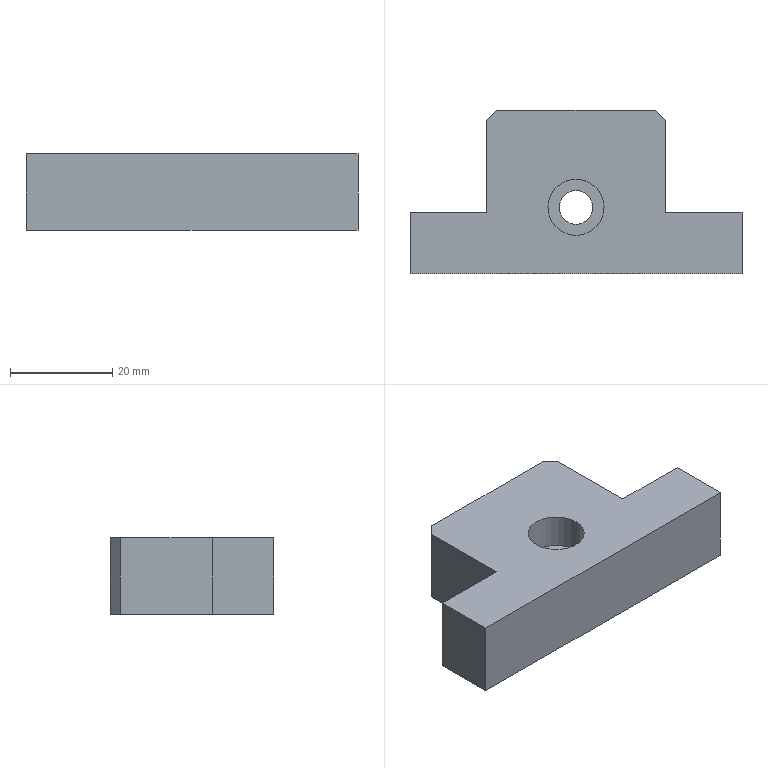Part | STEP file | PN_0005 | 1 solid | 17 faces | box 65 x 32 x 15 mm | volume 21213 mm3 | plane 13 | cylinder 4 | commonest cylinder face diameters 6.6 x2 11 x2
STEP:
#1=CARTESIAN_POINT('',(0.,0.,0.));
#2=DIRECTION('',(0.,0.,1.));
#3=DIRECTION('',(1.,0.,0.));
#4=AXIS2_PLACEMENT_3D('',#1,#2,#3);
#5=CARTESIAN_POINT('',(38.,13.,8.2));
#6=VERTEX_POINT('',#5);
#7=CARTESIAN_POINT('',(38.,13.,15.));
#8=VERTEX_POINT('',#7);
#9=CARTESIAN_POINT('',(38.,13.,15.));
#10=DIRECTION('',(0.,0.,1.));
#11=VECTOR('',#10,1.);
#12=LINE('',#9,#11);
#13=CARTESIAN_POINT('',(32.5,13.,15.));
#14=DIRECTION('',(0.,0.,1.));
#15=DIRECTION('',(1.,0.,0.));
#16=AXIS2_PLACEMENT_3D('',#13,#14,#15);
#17=CYLINDRICAL_SURFACE('',#16,5.5);
#18=CARTESIAN_POINT('',(6.283,0.));
#19=DIRECTION('',(0.,1.));
#20=VECTOR('',#19,1.);
#21=LINE('',#18,#20);
#22=(GEOMETRIC_REPRESENTATION_CONTEXT(2)PARAMETRIC_REPRESENTATION_CONTEXT()REPRESENTATION_CONTEXT('',''));
#23=DEFINITIONAL_REPRESENTATION('',(#21),#22);
#24=PCURVE('',#17,#23);
#25=CARTESIAN_POINT('',(32.5,13.,15.));
#26=DIRECTION('',(0.,0.,1.));
#27=DIRECTION('',(1.,0.,0.));
#28=AXIS2_PLACEMENT_3D('',#25,#26,#27);
#29=CYLINDRICAL_SURFACE('',#28,5.5);
#30=CARTESIAN_POINT('',(0.,0.));
#31=DIRECTION('',(0.,1.));
#32=VECTOR('',#31,1.);
#33=LINE('',#30,#32);
#34=(GEOMETRIC_REPRESENTATION_CONTEXT(2)PARAMETRIC_REPRESENTATION_CONTEXT()REPRESENTATION_CONTEXT('',''));
#35=DEFINITIONAL_REPRESENTATION('',(#33),#34);
#36=PCURVE('',#29,#35);
#37=SURFACE_CURVE('',#12,(#24,#36),.PCURVE_S1.);
#38=EDGE_CURVE('',#6,#8,#37,.T.);
#39=ORIENTED_EDGE('',*,*,#38,.T.);
#40=CARTESIAN_POINT('',(27.,13.,15.));
#41=VERTEX_POINT('',#40);
#42=CARTESIAN_POINT('',(32.5,13.,15.));
#43=DIRECTION('',(0.,0.,1.));
#44=DIRECTION('',(1.,0.,0.));
#45=AXIS2_PLACEMENT_3D('',#42,#43,#44);
#46=CIRCLE('',#45,5.5);
#47=CARTESIAN_POINT('',(0.,0.));
#48=DIRECTION('',(1.,0.));
#49=VECTOR('',#48,1.);
#50=LINE('',#47,#49);
#51=(GEOMETRIC_REPRESENTATION_CONTEXT(2)PARAMETRIC_REPRESENTATION_CONTEXT()REPRESENTATION_CONTEXT('',''));
#52=DEFINITIONAL_REPRESENTATION('',(#50),#51);
#53=PCURVE('',#17,#52);
#54=CARTESIAN_POINT('',(0.,12.,15.));
#55=DIRECTION('',(0.,0.,-1.));
#56=DIRECTION('',(-1.,0.,0.));
#57=AXIS2_PLACEMENT_3D('',#54,#55,#56);
#58=PLANE('',#57);
#59=CARTESIAN_POINT('',(-38.,1.));
#60=CARTESIAN_POINT('',(-38.,10.526));
#61=CARTESIAN_POINT('',(-29.75,5.763));
#62=CARTESIAN_POINT('',(-21.5,1.));
#63=CARTESIAN_POINT('',(-29.75,-3.763));
#64=CARTESIAN_POINT('',(-38.,-8.526));
#65=CARTESIAN_POINT('',(-38.,1.));
#66=(BOUNDED_CURVE()B_SPLINE_CURVE(2,(#59,#60,#61,#62,#63,#64,#65),.UNSPECIFIED.,.T.,.F.)B_SPLINE_CURVE_WITH_KNOTS((1,2,2,2,2,1),(-2.094,0.,2.094,4.189,6.283,8.378),.UNSPECIFIED.)CURVE()GEOMETRIC_REPRESENTATION_ITEM()RATIONAL_B_SPLINE_CURVE((1.,0.5,1.,0.5,1.,0.5,1.))REPRESENTATION_ITEM(''));
#67=(GEOMETRIC_REPRESENTATION_CONTEXT(2)PARAMETRIC_REPRESENTATION_CONTEXT()REPRESENTATION_CONTEXT('',''));
#68=DEFINITIONAL_REPRESENTATION('',(#66),#67);
#69=PCURVE('',#58,#68);
#70=SURFACE_CURVE('',#46,(#53,#69),.PCURVE_S1.);
#71=EDGE_CURVE('',#41,#8,#70,.T.);
#72=ORIENTED_EDGE('',*,*,#71,.F.);
#73=CARTESIAN_POINT('',(27.,13.,8.2));
#74=VERTEX_POINT('',#73);
#75=CARTESIAN_POINT('',(27.,13.,15.));
#76=DIRECTION('',(0.,0.,1.));
#77=VECTOR('',#76,1.);
#78=LINE('',#75,#77);
#79=CARTESIAN_POINT('',(3.142,0.));
#80=DIRECTION('',(0.,1.));
#81=VECTOR('',#80,1.);
#82=LINE('',#79,#81);
#83=(GEOMETRIC_REPRESENTATION_CONTEXT(2)PARAMETRIC_REPRESENTATION_CONTEXT()REPRESENTATION_CONTEXT('',''));
#84=DEFINITIONAL_REPRESENTATION('',(#82),#83);
#85=PCURVE('',#17,#84);
#86=CARTESIAN_POINT('',(3.142,0.));
#87=DIRECTION('',(0.,1.));
#88=VECTOR('',#87,1.);
#89=LINE('',#86,#88);
#90=(GEOMETRIC_REPRESENTATION_CONTEXT(2)PARAMETRIC_REPRESENTATION_CONTEXT()REPRESENTATION_CONTEXT('',''));
#91=DEFINITIONAL_REPRESENTATION('',(#89),#90);
#92=PCURVE('',#29,#91);
#93=SURFACE_CURVE('',#78,(#85,#92),.PCURVE_S1.);
#94=EDGE_CURVE('',#74,#41,#93,.T.);
#95=ORIENTED_EDGE('',*,*,#94,.F.);
#96=CARTESIAN_POINT('',(32.5,13.,8.2));
#97=DIRECTION('',(0.,0.,1.));
#98=DIRECTION('',(1.,0.,0.));
#99=AXIS2_PLACEMENT_3D('',#96,#97,#98);
#100=CIRCLE('',#99,5.5);
#101=CARTESIAN_POINT('',(0.,-6.8));
#102=DIRECTION('',(1.,0.));
#103=VECTOR('',#102,1.);
#104=LINE('',#101,#103);
#105=(GEOMETRIC_REPRESENTATION_CONTEXT(2)PARAMETRIC_REPRESENTATION_CONTEXT()REPRESENTATION_CONTEXT('',''));
#106=DEFINITIONAL_REPRESENTATION('',(#104),#105);
#107=PCURVE('',#17,#106);
#108=CARTESIAN_POINT('',(35.8,13.,8.2));
#109=DIRECTION('',(0.,0.,-1.));
#110=DIRECTION('',(-1.,0.,0.));
#111=AXIS2_PLACEMENT_3D('',#108,#109,#110);
#112=PLANE('',#111);
#113=CARTESIAN_POINT('',(-2.2,0.));
#114=CARTESIAN_POINT('',(-2.2,9.526));
#115=CARTESIAN_POINT('',(6.05,4.763));
#116=CARTESIAN_POINT('',(14.3,0.));
#117=CARTESIAN_POINT('',(6.05,-4.763));
#118=CARTESIAN_POINT('',(-2.2,-9.526));
#119=CARTESIAN_POINT('',(-2.2,0.));
#120=(BOUNDED_CURVE()B_SPLINE_CURVE(2,(#113,#114,#115,#116,#117,#118,#119),.UNSPECIFIED.,.T.,.F.)B_SPLINE_CURVE_WITH_KNOTS((1,2,2,2,2,1),(-2.094,0.,2.094,4.189,6.283,8.378),.UNSPECIFIED.)CURVE()GEOMETRIC_REPRESENTATION_ITEM()RATIONAL_B_SPLINE_CURVE((1.,0.5,1.,0.5,1.,0.5,1.))REPRESENTATION_ITEM(''));
#121=(GEOMETRIC_REPRESENTATION_CONTEXT(2)PARAMETRIC_REPRESENTATION_CONTEXT()REPRESENTATION_CONTEXT('',''));
#122=DEFINITIONAL_REPRESENTATION('',(#120),#121);
#123=PCURVE('',#112,#122);
#124=SURFACE_CURVE('',#100,(#107,#123),.PCURVE_S1.);
#125=EDGE_CURVE('',#74,#6,#124,.T.);
#126=ORIENTED_EDGE('',*,*,#125,.T.);
#127=EDGE_LOOP('',(#39,#72,#95,#126));
#128=FACE_BOUND('',#127,.F.);
#129=ADVANCED_FACE('',(#128),#17,.F.);
#130=CARTESIAN_POINT('',(35.8,13.,0.));
#131=VERTEX_POINT('',#130);
#132=CARTESIAN_POINT('',(35.8,13.,8.2));
#133=VERTEX_POINT('',#132);
#134=CARTESIAN_POINT('',(35.8,13.,15.));
#135=DIRECTION('',(0.,0.,1.));
#136=VECTOR('',#135,1.);
#137=LINE('',#134,#136);
#138=CARTESIAN_POINT('',(32.5,13.,15.));
#139=DIRECTION('',(0.,0.,1.));
#140=DIRECTION('',(1.,0.,0.));
#141=AXIS2_PLACEMENT_3D('',#138,#139,#140);
#142=CYLINDRICAL_SURFACE('',#141,3.3);
#143=CARTESIAN_POINT('',(6.283,0.));
#144=DIRECTION('',(0.,1.));
#145=VECTOR('',#144,1.);
#146=LINE('',#143,#145);
#147=(GEOMETRIC_REPRESENTATION_CONTEXT(2)PARAMETRIC_REPRESENTATION_CONTEXT()REPRESENTATION_CONTEXT('',''));
#148=DEFINITIONAL_REPRESENTATION('',(#146),#147);
#149=PCURVE('',#142,#148);
#150=CARTESIAN_POINT('',(32.5,13.,15.));
#151=DIRECTION('',(0.,0.,1.));
#152=DIRECTION('',(1.,0.,0.));
#153=AXIS2_PLACEMENT_3D('',#150,#151,#152);
#154=CYLINDRICAL_SURFACE('',#153,3.3);
#155=CARTESIAN_POINT('',(0.,0.));
#156=DIRECTION('',(0.,1.));
#157=VECTOR('',#156,1.);
#158=LINE('',#155,#157);
#159=(GEOMETRIC_REPRESENTATION_CONTEXT(2)PARAMETRIC_REPRESENTATION_CONTEXT()REPRESENTATION_CONTEXT('',''));
#160=DEFINITIONAL_REPRESENTATION('',(#158),#159);
#161=PCURVE('',#154,#160);
#162=SURFACE_CURVE('',#137,(#149,#161),.PCURVE_S1.);
#163=EDGE_CURVE('',#131,#133,#162,.T.);
#164=ORIENTED_EDGE('',*,*,#163,.T.);
#165=CARTESIAN_POINT('',(29.2,13.,8.2));
#166=VERTEX_POINT('',#165);
#167=CARTESIAN_POINT('',(32.5,13.,8.2));
#168=DIRECTION('',(0.,0.,1.));
#169=DIRECTION('',(1.,0.,0.));
#170=AXIS2_PLACEMENT_3D('',#167,#168,#169);
#171=CIRCLE('',#170,3.3);
#172=CARTESIAN_POINT('',(0.,-6.8));
#173=DIRECTION('',(1.,0.));
#174=VECTOR('',#173,1.);
#175=LINE('',#172,#174);
#176=(GEOMETRIC_REPRESENTATION_CONTEXT(2)PARAMETRIC_REPRESENTATION_CONTEXT()REPRESENTATION_CONTEXT('',''));
#177=DEFINITIONAL_REPRESENTATION('',(#175),#176);
#178=PCURVE('',#142,#177);
#179=CARTESIAN_POINT('',(0.,0.));
#180=CARTESIAN_POINT('',(0.,5.716));
#181=CARTESIAN_POINT('',(4.95,2.858));
#182=CARTESIAN_POINT('',(9.9,0.));
#183=CARTESIAN_POINT('',(4.95,-2.858));
#184=CARTESIAN_POINT('',(0.,-5.716));
#185=CARTESIAN_POINT('',(0.,0.));
#186=(BOUNDED_CURVE()B_SPLINE_CURVE(2,(#179,#180,#181,#182,#183,#184,#185),.UNSPECIFIED.,.T.,.F.)B_SPLINE_CURVE_WITH_KNOTS((1,2,2,2,2,1),(-2.094,0.,2.094,4.189,6.283,8.378),.UNSPECIFIED.)CURVE()GEOMETRIC_REPRESENTATION_ITEM()RATIONAL_B_SPLINE_CURVE((1.,0.5,1.,0.5,1.,0.5,1.))REPRESENTATION_ITEM(''));
#187=(GEOMETRIC_REPRESENTATION_CONTEXT(2)PARAMETRIC_REPRESENTATION_CONTEXT()REPRESENTATION_CONTEXT('',''));
#188=DEFINITIONAL_REPRESENTATION('',(#186),#187);
#189=PCURVE('',#112,#188);
#190=SURFACE_CURVE('',#171,(#178,#189),.PCURVE_S1.);
#191=EDGE_CURVE('',#166,#133,#190,.T.);
#192=ORIENTED_EDGE('',*,*,#191,.F.);
#193=CARTESIAN_POINT('',(29.2,13.,0.));
#194=VERTEX_POINT('',#193);
#195=CARTESIAN_POINT('',(29.2,13.,15.));
#196=DIRECTION('',(0.,0.,1.));
#197=VECTOR('',#196,1.);
#198=LINE('',#195,#197);
#199=CARTESIAN_POINT('',(3.142,0.));
#200=DIRECTION('',(0.,1.));
#201=VECTOR('',#200,1.);
#202=LINE('',#199,#201);
#203=(GEOMETRIC_REPRESENTATION_CONTEXT(2)PARAMETRIC_REPRESENTATION_CONTEXT()REPRESENTATION_CONTEXT('',''));
#204=DEFINITIONAL_REPRESENTATION('',(#202),#203);
#205=PCURVE('',#142,#204);
#206=CARTESIAN_POINT('',(3.142,0.));
#207=DIRECTION('',(0.,1.));
#208=VECTOR('',#207,1.);
#209=LINE('',#206,#208);
#210=(GEOMETRIC_REPRESENTATION_CONTEXT(2)PARAMETRIC_REPRESENTATION_CONTEXT()REPRESENTATION_CONTEXT('',''));
#211=DEFINITIONAL_REPRESENTATION('',(#209),#210);
#212=PCURVE('',#154,#211);
#213=SURFACE_CURVE('',#198,(#205,#212),.PCURVE_S1.);
#214=EDGE_CURVE('',#194,#166,#213,.T.);
#215=ORIENTED_EDGE('',*,*,#214,.F.);
#216=CARTESIAN_POINT('',(32.5,13.,0.));
#217=DIRECTION('',(0.,0.,1.));
#218=DIRECTION('',(1.,0.,0.));
#219=AXIS2_PLACEMENT_3D('',#216,#217,#218);
#220=CIRCLE('',#219,3.3);
#221=CARTESIAN_POINT('',(0.,-15.));
#222=DIRECTION('',(1.,0.));
#223=VECTOR('',#222,1.);
#224=LINE('',#221,#223);
#225=(GEOMETRIC_REPRESENTATION_CONTEXT(2)PARAMETRIC_REPRESENTATION_CONTEXT()REPRESENTATION_CONTEXT('',''));
#226=DEFINITIONAL_REPRESENTATION('',(#224),#225);
#227=PCURVE('',#142,#226);
#228=CARTESIAN_POINT('',(0.,12.,0.));
#229=DIRECTION('',(0.,0.,-1.));
#230=DIRECTION('',(-1.,0.,0.));
#231=AXIS2_PLACEMENT_3D('',#228,#229,#230);
#232=PLANE('',#231);
#233=CARTESIAN_POINT('',(-35.8,1.));
#234=CARTESIAN_POINT('',(-35.8,6.716));
#235=CARTESIAN_POINT('',(-30.85,3.858));
#236=CARTESIAN_POINT('',(-25.9,1.));
#237=CARTESIAN_POINT('',(-30.85,-1.858));
#238=CARTESIAN_POINT('',(-35.8,-4.716));
#239=CARTESIAN_POINT('',(-35.8,1.));
#240=(BOUNDED_CURVE()B_SPLINE_CURVE(2,(#233,#234,#235,#236,#237,#238,#239),.UNSPECIFIED.,.T.,.F.)B_SPLINE_CURVE_WITH_KNOTS((1,2,2,2,2,1),(-2.094,0.,2.094,4.189,6.283,8.378),.UNSPECIFIED.)CURVE()GEOMETRIC_REPRESENTATION_ITEM()RATIONAL_B_SPLINE_CURVE((1.,0.5,1.,0.5,1.,0.5,1.))REPRESENTATION_ITEM(''));
#241=(GEOMETRIC_REPRESENTATION_CONTEXT(2)PARAMETRIC_REPRESENTATION_CONTEXT()REPRESENTATION_CONTEXT('',''));
#242=DEFINITIONAL_REPRESENTATION('',(#240),#241);
#243=PCURVE('',#232,#242);
#244=SURFACE_CURVE('',#220,(#227,#243),.PCURVE_S1.);
#245=EDGE_CURVE('',#194,#131,#244,.T.);
#246=ORIENTED_EDGE('',*,*,#245,.T.);
#247=EDGE_LOOP('',(#164,#192,#215,#246));
#248=FACE_BOUND('',#247,.F.);
#249=ADVANCED_FACE('',(#248),#142,.F.);
#250=CARTESIAN_POINT('',(0.,12.,0.));
#251=VERTEX_POINT('',#250);
#252=CARTESIAN_POINT('',(0.,0.,0.));
#253=VERTEX_POINT('',#252);
#254=CARTESIAN_POINT('',(0.,0.,0.));
#255=DIRECTION('',(0.,-1.,0.));
#256=VECTOR('',#255,1.);
#257=LINE('',#254,#256);
#258=CARTESIAN_POINT('',(0.,0.,15.));
#259=DIRECTION('',(1.,0.,0.));
#260=DIRECTION('',(0.,0.,-1.));
#261=AXIS2_PLACEMENT_3D('',#258,#259,#260);
#262=PLANE('',#261);
#263=CARTESIAN_POINT('',(15.,0.));
#264=DIRECTION('',(0.,-1.));
#265=VECTOR('',#264,1.);
#266=LINE('',#263,#265);
#267=(GEOMETRIC_REPRESENTATION_CONTEXT(2)PARAMETRIC_REPRESENTATION_CONTEXT()REPRESENTATION_CONTEXT('',''));
#268=DEFINITIONAL_REPRESENTATION('',(#266),#267);
#269=PCURVE('',#262,#268);
#270=CARTESIAN_POINT('',(0.,-12.));
#271=DIRECTION('',(0.,-1.));
#272=VECTOR('',#271,1.);
#273=LINE('',#270,#272);
#274=(GEOMETRIC_REPRESENTATION_CONTEXT(2)PARAMETRIC_REPRESENTATION_CONTEXT()REPRESENTATION_CONTEXT('',''));
#275=DEFINITIONAL_REPRESENTATION('',(#273),#274);
#276=PCURVE('',#232,#275);
#277=SURFACE_CURVE('',#257,(#269,#276),.PCURVE_S1.);
#278=EDGE_CURVE('',#251,#253,#277,.T.);
#279=ORIENTED_EDGE('',*,*,#278,.T.);
#280=CARTESIAN_POINT('',(0.,0.,15.));
#281=VERTEX_POINT('',#280);
#282=CARTESIAN_POINT('',(0.,0.,15.));
#283=DIRECTION('',(0.,0.,-1.));
#284=VECTOR('',#283,1.);
#285=LINE('',#282,#284);
#286=CARTESIAN_POINT('',(0.,0.));
#287=DIRECTION('',(1.,0.));
#288=VECTOR('',#287,1.);
#289=LINE('',#286,#288);
#290=(GEOMETRIC_REPRESENTATION_CONTEXT(2)PARAMETRIC_REPRESENTATION_CONTEXT()REPRESENTATION_CONTEXT('',''));
#291=DEFINITIONAL_REPRESENTATION('',(#289),#290);
#292=PCURVE('',#262,#291);
#293=CARTESIAN_POINT('',(0.,0.,15.));
#294=DIRECTION('',(0.,1.,0.));
#295=DIRECTION('',(-1.,0.,0.));
#296=AXIS2_PLACEMENT_3D('',#293,#294,#295);
#297=PLANE('',#296);
#298=CARTESIAN_POINT('',(0.,0.));
#299=DIRECTION('',(0.,-1.));
#300=VECTOR('',#299,1.);
#301=LINE('',#298,#300);
#302=(GEOMETRIC_REPRESENTATION_CONTEXT(2)PARAMETRIC_REPRESENTATION_CONTEXT()REPRESENTATION_CONTEXT('',''));
#303=DEFINITIONAL_REPRESENTATION('',(#301),#302);
#304=PCURVE('',#297,#303);
#305=SURFACE_CURVE('',#285,(#292,#304),.PCURVE_S1.);
#306=EDGE_CURVE('',#281,#253,#305,.T.);
#307=ORIENTED_EDGE('',*,*,#306,.F.);
#308=CARTESIAN_POINT('',(0.,12.,15.));
#309=VERTEX_POINT('',#308);
#310=CARTESIAN_POINT('',(0.,0.,15.));
#311=DIRECTION('',(0.,-1.,0.));
#312=VECTOR('',#311,1.);
#313=LINE('',#310,#312);
#314=CARTESIAN_POINT('',(0.,0.));
#315=DIRECTION('',(0.,-1.));
#316=VECTOR('',#315,1.);
#317=LINE('',#314,#316);
#318=(GEOMETRIC_REPRESENTATION_CONTEXT(2)PARAMETRIC_REPRESENTATION_CONTEXT()REPRESENTATION_CONTEXT('',''));
#319=DEFINITIONAL_REPRESENTATION('',(#317),#318);
#320=PCURVE('',#262,#319);
#321=CARTESIAN_POINT('',(0.,-12.));
#322=DIRECTION('',(0.,-1.));
#323=VECTOR('',#322,1.);
#324=LINE('',#321,#323);
#325=(GEOMETRIC_REPRESENTATION_CONTEXT(2)PARAMETRIC_REPRESENTATION_CONTEXT()REPRESENTATION_CONTEXT('',''));
#326=DEFINITIONAL_REPRESENTATION('',(#324),#325);
#327=PCURVE('',#58,#326);
#328=SURFACE_CURVE('',#313,(#320,#327),.PCURVE_S1.);
#329=EDGE_CURVE('',#309,#281,#328,.T.);
#330=ORIENTED_EDGE('',*,*,#329,.F.);
#331=CARTESIAN_POINT('',(0.,12.,15.));
#332=DIRECTION('',(0.,0.,-1.));
#333=VECTOR('',#332,1.);
#334=LINE('',#331,#333);
#335=CARTESIAN_POINT('',(0.,12.));
#336=DIRECTION('',(1.,0.));
#337=VECTOR('',#336,1.);
#338=LINE('',#335,#337);
#339=(GEOMETRIC_REPRESENTATION_CONTEXT(2)PARAMETRIC_REPRESENTATION_CONTEXT()REPRESENTATION_CONTEXT('',''));
#340=DEFINITIONAL_REPRESENTATION('',(#338),#339);
#341=PCURVE('',#262,#340);
#342=CARTESIAN_POINT('',(0.,12.,15.));
#343=DIRECTION('',(0.,-1.,0.));
#344=DIRECTION('',(0.,0.,-1.));
#345=AXIS2_PLACEMENT_3D('',#342,#343,#344);
#346=PLANE('',#345);
#347=CARTESIAN_POINT('',(0.,0.));
#348=DIRECTION('',(1.,0.));
#349=VECTOR('',#348,1.);
#350=LINE('',#347,#349);
#351=(GEOMETRIC_REPRESENTATION_CONTEXT(2)PARAMETRIC_REPRESENTATION_CONTEXT()REPRESENTATION_CONTEXT('',''));
#352=DEFINITIONAL_REPRESENTATION('',(#350),#351);
#353=PCURVE('',#346,#352);
#354=SURFACE_CURVE('',#334,(#341,#353),.PCURVE_S1.);
#355=EDGE_CURVE('',#309,#251,#354,.T.);
#356=ORIENTED_EDGE('',*,*,#355,.T.);
#357=EDGE_LOOP('',(#279,#307,#330,#356));
#358=FACE_BOUND('',#357,.T.);
#359=ADVANCED_FACE('',(#358),#262,.F.);
#360=CARTESIAN_POINT('',(65.,0.,0.));
#361=VERTEX_POINT('',#360);
#362=CARTESIAN_POINT('',(0.,0.,0.));
#363=DIRECTION('',(1.,0.,0.));
#364=VECTOR('',#363,1.);
#365=LINE('',#362,#364);
#366=CARTESIAN_POINT('',(0.,-15.));
#367=DIRECTION('',(-1.,0.));
#368=VECTOR('',#367,1.);
#369=LINE('',#366,#368);
#370=(GEOMETRIC_REPRESENTATION_CONTEXT(2)PARAMETRIC_REPRESENTATION_CONTEXT()REPRESENTATION_CONTEXT('',''));
#371=DEFINITIONAL_REPRESENTATION('',(#369),#370);
#372=PCURVE('',#297,#371);
#373=CARTESIAN_POINT('',(0.,-12.));
#374=DIRECTION('',(-1.,0.));
#375=VECTOR('',#374,1.);
#376=LINE('',#373,#375);
#377=(GEOMETRIC_REPRESENTATION_CONTEXT(2)PARAMETRIC_REPRESENTATION_CONTEXT()REPRESENTATION_CONTEXT('',''));
#378=DEFINITIONAL_REPRESENTATION('',(#376),#377);
#379=PCURVE('',#232,#378);
#380=SURFACE_CURVE('',#365,(#372,#379),.PCURVE_S1.);
#381=EDGE_CURVE('',#253,#361,#380,.T.);
#382=ORIENTED_EDGE('',*,*,#381,.T.);
#383=CARTESIAN_POINT('',(65.,0.,15.));
#384=VERTEX_POINT('',#383);
#385=CARTESIAN_POINT('',(65.,0.,15.));
#386=DIRECTION('',(0.,0.,-1.));
#387=VECTOR('',#386,1.);
#388=LINE('',#385,#387);
#389=CARTESIAN_POINT('',(-65.,0.));
#390=DIRECTION('',(0.,-1.));
#391=VECTOR('',#390,1.);
#392=LINE('',#389,#391);
#393=(GEOMETRIC_REPRESENTATION_CONTEXT(2)PARAMETRIC_REPRESENTATION_CONTEXT()REPRESENTATION_CONTEXT('',''));
#394=DEFINITIONAL_REPRESENTATION('',(#392),#393);
#395=PCURVE('',#297,#394);
#396=CARTESIAN_POINT('',(65.,0.,15.));
#397=DIRECTION('',(-1.,0.,0.));
#398=DIRECTION('',(0.,-1.,0.));
#399=AXIS2_PLACEMENT_3D('',#396,#397,#398);
#400=PLANE('',#399);
#401=CARTESIAN_POINT('',(0.,0.));
#402=DIRECTION('',(0.,-1.));
#403=VECTOR('',#402,1.);
#404=LINE('',#401,#403);
#405=(GEOMETRIC_REPRESENTATION_CONTEXT(2)PARAMETRIC_REPRESENTATION_CONTEXT()REPRESENTATION_CONTEXT('',''));
#406=DEFINITIONAL_REPRESENTATION('',(#404),#405);
#407=PCURVE('',#400,#406);
#408=SURFACE_CURVE('',#388,(#395,#407),.PCURVE_S1.);
#409=EDGE_CURVE('',#384,#361,#408,.T.);
#410=ORIENTED_EDGE('',*,*,#409,.F.);
#411=CARTESIAN_POINT('',(0.,0.,15.));
#412=DIRECTION('',(1.,0.,0.));
#413=VECTOR('',#412,1.);
#414=LINE('',#411,#413);
#415=CARTESIAN_POINT('',(0.,0.));
#416=DIRECTION('',(-1.,0.));
#417=VECTOR('',#416,1.);
#418=LINE('',#415,#417);
#419=(GEOMETRIC_REPRESENTATION_CONTEXT(2)PARAMETRIC_REPRESENTATION_CONTEXT()REPRESENTATION_CONTEXT('',''));
#420=DEFINITIONAL_REPRESENTATION('',(#418),#419);
#421=PCURVE('',#297,#420);
#422=CARTESIAN_POINT('',(0.,-12.));
#423=DIRECTION('',(-1.,0.));
#424=VECTOR('',#423,1.);
#425=LINE('',#422,#424);
#426=(GEOMETRIC_REPRESENTATION_CONTEXT(2)PARAMETRIC_REPRESENTATION_CONTEXT()REPRESENTATION_CONTEXT('',''));
#427=DEFINITIONAL_REPRESENTATION('',(#425),#426);
#428=PCURVE('',#58,#427);
#429=SURFACE_CURVE('',#414,(#421,#428),.PCURVE_S1.);
#430=EDGE_CURVE('',#281,#384,#429,.T.);
#431=ORIENTED_EDGE('',*,*,#430,.F.);
#432=ORIENTED_EDGE('',*,*,#306,.T.);
#433=EDGE_LOOP('',(#382,#410,#431,#432));
#434=FACE_BOUND('',#433,.T.);
#435=ADVANCED_FACE('',(#434),#297,.F.);
#436=CARTESIAN_POINT('',(65.,12.,0.));
#437=VERTEX_POINT('',#436);
#438=CARTESIAN_POINT('',(65.,0.,0.));
#439=DIRECTION('',(0.,1.,0.));
#440=VECTOR('',#439,1.);
#441=LINE('',#438,#440);
#442=CARTESIAN_POINT('',(0.,-15.));
#443=DIRECTION('',(-1.,0.));
#444=VECTOR('',#443,1.);
#445=LINE('',#442,#444);
#446=(GEOMETRIC_REPRESENTATION_CONTEXT(2)PARAMETRIC_REPRESENTATION_CONTEXT()REPRESENTATION_CONTEXT('',''));
#447=DEFINITIONAL_REPRESENTATION('',(#445),#446);
#448=PCURVE('',#400,#447);
#449=CARTESIAN_POINT('',(-65.,-12.));
#450=DIRECTION('',(0.,1.));
#451=VECTOR('',#450,1.);
#452=LINE('',#449,#451);
#453=(GEOMETRIC_REPRESENTATION_CONTEXT(2)PARAMETRIC_REPRESENTATION_CONTEXT()REPRESENTATION_CONTEXT('',''));
#454=DEFINITIONAL_REPRESENTATION('',(#452),#453);
#455=PCURVE('',#232,#454);
#456=SURFACE_CURVE('',#441,(#448,#455),.PCURVE_S1.);
#457=EDGE_CURVE('',#361,#437,#456,.T.);
#458=ORIENTED_EDGE('',*,*,#457,.T.);
#459=CARTESIAN_POINT('',(65.,12.,15.));
#460=VERTEX_POINT('',#459);
#461=CARTESIAN_POINT('',(65.,12.,15.));
#462=DIRECTION('',(0.,0.,-1.));
#463=VECTOR('',#462,1.);
#464=LINE('',#461,#463);
#465=CARTESIAN_POINT('',(-12.,0.));
#466=DIRECTION('',(0.,-1.));
#467=VECTOR('',#466,1.);
#468=LINE('',#465,#467);
#469=(GEOMETRIC_REPRESENTATION_CONTEXT(2)PARAMETRIC_REPRESENTATION_CONTEXT()REPRESENTATION_CONTEXT('',''));
#470=DEFINITIONAL_REPRESENTATION('',(#468),#469);
#471=PCURVE('',#400,#470);
#472=CARTESIAN_POINT('',(65.,12.,15.));
#473=DIRECTION('',(0.,-1.,0.));
#474=DIRECTION('',(1.,0.,0.));
#475=AXIS2_PLACEMENT_3D('',#472,#473,#474);
#476=PLANE('',#475);
#477=CARTESIAN_POINT('',(0.,0.));
#478=DIRECTION('',(0.,-1.));
#479=VECTOR('',#478,1.);
#480=LINE('',#477,#479);
#481=(GEOMETRIC_REPRESENTATION_CONTEXT(2)PARAMETRIC_REPRESENTATION_CONTEXT()REPRESENTATION_CONTEXT('',''));
#482=DEFINITIONAL_REPRESENTATION('',(#480),#481);
#483=PCURVE('',#476,#482);
#484=SURFACE_CURVE('',#464,(#471,#483),.PCURVE_S1.);
#485=EDGE_CURVE('',#460,#437,#484,.T.);
#486=ORIENTED_EDGE('',*,*,#485,.F.);
#487=CARTESIAN_POINT('',(65.,0.,15.));
#488=DIRECTION('',(0.,1.,0.));
#489=VECTOR('',#488,1.);
#490=LINE('',#487,#489);
#491=CARTESIAN_POINT('',(0.,0.));
#492=DIRECTION('',(-1.,0.));
#493=VECTOR('',#492,1.);
#494=LINE('',#491,#493);
#495=(GEOMETRIC_REPRESENTATION_CONTEXT(2)PARAMETRIC_REPRESENTATION_CONTEXT()REPRESENTATION_CONTEXT('',''));
#496=DEFINITIONAL_REPRESENTATION('',(#494),#495);
#497=PCURVE('',#400,#496);
#498=CARTESIAN_POINT('',(-65.,-12.));
#499=DIRECTION('',(0.,1.));
#500=VECTOR('',#499,1.);
#501=LINE('',#498,#500);
#502=(GEOMETRIC_REPRESENTATION_CONTEXT(2)PARAMETRIC_REPRESENTATION_CONTEXT()REPRESENTATION_CONTEXT('',''));
#503=DEFINITIONAL_REPRESENTATION('',(#501),#502);
#504=PCURVE('',#58,#503);
#505=SURFACE_CURVE('',#490,(#497,#504),.PCURVE_S1.);
#506=EDGE_CURVE('',#384,#460,#505,.T.);
#507=ORIENTED_EDGE('',*,*,#506,.F.);
#508=ORIENTED_EDGE('',*,*,#409,.T.);
#509=EDGE_LOOP('',(#458,#486,#507,#508));
#510=FACE_BOUND('',#509,.T.);
#511=ADVANCED_FACE('',(#510),#400,.F.);
#512=CARTESIAN_POINT('',(50.,12.,0.));
#513=VERTEX_POINT('',#512);
#514=CARTESIAN_POINT('',(65.,12.,0.));
#515=DIRECTION('',(-1.,0.,0.));
#516=VECTOR('',#515,1.);
#517=LINE('',#514,#516);
#518=CARTESIAN_POINT('',(0.,-15.));
#519=DIRECTION('',(-1.,0.));
#520=VECTOR('',#519,1.);
#521=LINE('',#518,#520);
#522=(GEOMETRIC_REPRESENTATION_CONTEXT(2)PARAMETRIC_REPRESENTATION_CONTEXT()REPRESENTATION_CONTEXT('',''));
#523=DEFINITIONAL_REPRESENTATION('',(#521),#522);
#524=PCURVE('',#476,#523);
#525=CARTESIAN_POINT('',(-65.,0.));
#526=DIRECTION('',(1.,0.));
#527=VECTOR('',#526,1.);
#528=LINE('',#525,#527);
#529=(GEOMETRIC_REPRESENTATION_CONTEXT(2)PARAMETRIC_REPRESENTATION_CONTEXT()REPRESENTATION_CONTEXT('',''));
#530=DEFINITIONAL_REPRESENTATION('',(#528),#529);
#531=PCURVE('',#232,#530);
#532=SURFACE_CURVE('',#517,(#524,#531),.PCURVE_S1.);
#533=EDGE_CURVE('',#437,#513,#532,.T.);
#534=ORIENTED_EDGE('',*,*,#533,.T.);
#535=CARTESIAN_POINT('',(50.,12.,15.));
#536=VERTEX_POINT('',#535);
#537=CARTESIAN_POINT('',(50.,12.,15.));
#538=DIRECTION('',(0.,0.,-1.));
#539=VECTOR('',#538,1.);
#540=LINE('',#537,#539);
#541=CARTESIAN_POINT('',(-15.,0.));
#542=DIRECTION('',(0.,-1.));
#543=VECTOR('',#542,1.);
#544=LINE('',#541,#543);
#545=(GEOMETRIC_REPRESENTATION_CONTEXT(2)PARAMETRIC_REPRESENTATION_CONTEXT()REPRESENTATION_CONTEXT('',''));
#546=DEFINITIONAL_REPRESENTATION('',(#544),#545);
#547=PCURVE('',#476,#546);
#548=CARTESIAN_POINT('',(50.,12.,15.));
#549=DIRECTION('',(-1.,0.,0.));
#550=DIRECTION('',(0.,-1.,0.));
#551=AXIS2_PLACEMENT_3D('',#548,#549,#550);
#552=PLANE('',#551);
#553=CARTESIAN_POINT('',(0.,0.));
#554=DIRECTION('',(0.,-1.));
#555=VECTOR('',#554,1.);
#556=LINE('',#553,#555);
#557=(GEOMETRIC_REPRESENTATION_CONTEXT(2)PARAMETRIC_REPRESENTATION_CONTEXT()REPRESENTATION_CONTEXT('',''));
#558=DEFINITIONAL_REPRESENTATION('',(#556),#557);
#559=PCURVE('',#552,#558);
#560=SURFACE_CURVE('',#540,(#547,#559),.PCURVE_S1.);
#561=EDGE_CURVE('',#536,#513,#560,.T.);
#562=ORIENTED_EDGE('',*,*,#561,.F.);
#563=CARTESIAN_POINT('',(65.,12.,15.));
#564=DIRECTION('',(-1.,0.,0.));
#565=VECTOR('',#564,1.);
#566=LINE('',#563,#565);
#567=CARTESIAN_POINT('',(0.,0.));
#568=DIRECTION('',(-1.,0.));
#569=VECTOR('',#568,1.);
#570=LINE('',#567,#569);
#571=(GEOMETRIC_REPRESENTATION_CONTEXT(2)PARAMETRIC_REPRESENTATION_CONTEXT()REPRESENTATION_CONTEXT('',''));
#572=DEFINITIONAL_REPRESENTATION('',(#570),#571);
#573=PCURVE('',#476,#572);
#574=CARTESIAN_POINT('',(-65.,0.));
#575=DIRECTION('',(1.,0.));
#576=VECTOR('',#575,1.);
#577=LINE('',#574,#576);
#578=(GEOMETRIC_REPRESENTATION_CONTEXT(2)PARAMETRIC_REPRESENTATION_CONTEXT()REPRESENTATION_CONTEXT('',''));
#579=DEFINITIONAL_REPRESENTATION('',(#577),#578);
#580=PCURVE('',#58,#579);
#581=SURFACE_CURVE('',#566,(#573,#580),.PCURVE_S1.);
#582=EDGE_CURVE('',#460,#536,#581,.T.);
#583=ORIENTED_EDGE('',*,*,#582,.F.);
#584=ORIENTED_EDGE('',*,*,#485,.T.);
#585=EDGE_LOOP('',(#534,#562,#583,#584));
#586=FACE_BOUND('',#585,.T.);
#587=ADVANCED_FACE('',(#586),#476,.F.);
#588=CARTESIAN_POINT('',(50.,30.,0.));
#589=VERTEX_POINT('',#588);
#590=CARTESIAN_POINT('',(50.,12.,0.));
#591=DIRECTION('',(0.,1.,0.));
#592=VECTOR('',#591,1.);
#593=LINE('',#590,#592);
#594=CARTESIAN_POINT('',(0.,-15.));
#595=DIRECTION('',(-1.,0.));
#596=VECTOR('',#595,1.);
#597=LINE('',#594,#596);
#598=(GEOMETRIC_REPRESENTATION_CONTEXT(2)PARAMETRIC_REPRESENTATION_CONTEXT()REPRESENTATION_CONTEXT('',''));
#599=DEFINITIONAL_REPRESENTATION('',(#597),#598);
#600=PCURVE('',#552,#599);
#601=CARTESIAN_POINT('',(-50.,0.));
#602=DIRECTION('',(0.,1.));
#603=VECTOR('',#602,1.);
#604=LINE('',#601,#603);
#605=(GEOMETRIC_REPRESENTATION_CONTEXT(2)PARAMETRIC_REPRESENTATION_CONTEXT()REPRESENTATION_CONTEXT('',''));
#606=DEFINITIONAL_REPRESENTATION('',(#604),#605);
#607=PCURVE('',#232,#606);
#608=SURFACE_CURVE('',#593,(#600,#607),.PCURVE_S1.);
#609=EDGE_CURVE('',#513,#589,#608,.T.);
#610=ORIENTED_EDGE('',*,*,#609,.T.);
#611=CARTESIAN_POINT('',(50.,30.,15.));
#612=VERTEX_POINT('',#611);
#613=CARTESIAN_POINT('',(50.,30.,15.));
#614=DIRECTION('',(0.,0.,1.));
#615=VECTOR('',#614,1.);
#616=LINE('',#613,#615);
#617=CARTESIAN_POINT('',(-18.,0.));
#618=DIRECTION('',(0.,1.));
#619=VECTOR('',#618,1.);
#620=LINE('',#617,#619);
#621=(GEOMETRIC_REPRESENTATION_CONTEXT(2)PARAMETRIC_REPRESENTATION_CONTEXT()REPRESENTATION_CONTEXT('',''));
#622=DEFINITIONAL_REPRESENTATION('',(#620),#621);
#623=PCURVE('',#552,#622);
#624=CARTESIAN_POINT('',(48.,32.,15.));
#625=DIRECTION('',(-0.7071,-0.7071,0.));
#626=DIRECTION('',(0.7071,-0.7071,0.));
#627=AXIS2_PLACEMENT_3D('',#624,#625,#626);
#628=PLANE('',#627);
#629=CARTESIAN_POINT('',(2.828,0.));
#630=DIRECTION('',(0.,1.));
#631=VECTOR('',#630,1.);
#632=LINE('',#629,#631);
#633=(GEOMETRIC_REPRESENTATION_CONTEXT(2)PARAMETRIC_REPRESENTATION_CONTEXT()REPRESENTATION_CONTEXT('',''));
#634=DEFINITIONAL_REPRESENTATION('',(#632),#633);
#635=PCURVE('',#628,#634);
#636=SURFACE_CURVE('',#616,(#623,#635),.PCURVE_S1.);
#637=EDGE_CURVE('',#589,#612,#636,.T.);
#638=ORIENTED_EDGE('',*,*,#637,.T.);
#639=CARTESIAN_POINT('',(50.,12.,15.));
#640=DIRECTION('',(0.,1.,0.));
#641=VECTOR('',#640,1.);
#642=LINE('',#639,#641);
#643=CARTESIAN_POINT('',(0.,0.));
#644=DIRECTION('',(-1.,0.));
#645=VECTOR('',#644,1.);
#646=LINE('',#643,#645);
#647=(GEOMETRIC_REPRESENTATION_CONTEXT(2)PARAMETRIC_REPRESENTATION_CONTEXT()REPRESENTATION_CONTEXT('',''));
#648=DEFINITIONAL_REPRESENTATION('',(#646),#647);
#649=PCURVE('',#552,#648);
#650=CARTESIAN_POINT('',(-50.,0.));
#651=DIRECTION('',(0.,1.));
#652=VECTOR('',#651,1.);
#653=LINE('',#650,#652);
#654=(GEOMETRIC_REPRESENTATION_CONTEXT(2)PARAMETRIC_REPRESENTATION_CONTEXT()REPRESENTATION_CONTEXT('',''));
#655=DEFINITIONAL_REPRESENTATION('',(#653),#654);
#656=PCURVE('',#58,#655);
#657=SURFACE_CURVE('',#642,(#649,#656),.PCURVE_S1.);
#658=EDGE_CURVE('',#536,#612,#657,.T.);
#659=ORIENTED_EDGE('',*,*,#658,.F.);
#660=ORIENTED_EDGE('',*,*,#561,.T.);
#661=EDGE_LOOP('',(#610,#638,#659,#660));
#662=FACE_BOUND('',#661,.T.);
#663=ADVANCED_FACE('',(#662),#552,.F.);
#664=CARTESIAN_POINT('',(48.,32.,15.));
#665=VERTEX_POINT('',#664);
#666=CARTESIAN_POINT('',(17.,32.,15.));
#667=VERTEX_POINT('',#666);
#668=CARTESIAN_POINT('',(15.,32.,15.));
#669=DIRECTION('',(-1.,0.,0.));
#670=VECTOR('',#669,1.);
#671=LINE('',#668,#670);
#672=CARTESIAN_POINT('',(15.,32.,15.));
#673=DIRECTION('',(0.,-1.,0.));
#674=DIRECTION('',(1.,0.,0.));
#675=AXIS2_PLACEMENT_3D('',#672,#673,#674);
#676=PLANE('',#675);
#677=CARTESIAN_POINT('',(0.,0.));
#678=DIRECTION('',(-1.,0.));
#679=VECTOR('',#678,1.);
#680=LINE('',#677,#679);
#681=(GEOMETRIC_REPRESENTATION_CONTEXT(2)PARAMETRIC_REPRESENTATION_CONTEXT()REPRESENTATION_CONTEXT('',''));
#682=DEFINITIONAL_REPRESENTATION('',(#680),#681);
#683=PCURVE('',#676,#682);
#684=CARTESIAN_POINT('',(-15.,20.));
#685=DIRECTION('',(1.,0.));
#686=VECTOR('',#685,1.);
#687=LINE('',#684,#686);
#688=(GEOMETRIC_REPRESENTATION_CONTEXT(2)PARAMETRIC_REPRESENTATION_CONTEXT()REPRESENTATION_CONTEXT('',''));
#689=DEFINITIONAL_REPRESENTATION('',(#687),#688);
#690=PCURVE('',#58,#689);
#691=SURFACE_CURVE('',#671,(#683,#690),.PCURVE_S1.);
#692=EDGE_CURVE('',#665,#667,#691,.T.);
#693=ORIENTED_EDGE('',*,*,#692,.F.);
#694=CARTESIAN_POINT('',(48.,32.,0.));
#695=VERTEX_POINT('',#694);
#696=CARTESIAN_POINT('',(48.,32.,15.));
#697=DIRECTION('',(0.,0.,-1.));
#698=VECTOR('',#697,1.);
#699=LINE('',#696,#698);
#700=CARTESIAN_POINT('',(33.,0.));
#701=DIRECTION('',(0.,-1.));
#702=VECTOR('',#701,1.);
#703=LINE('',#700,#702);
#704=(GEOMETRIC_REPRESENTATION_CONTEXT(2)PARAMETRIC_REPRESENTATION_CONTEXT()REPRESENTATION_CONTEXT('',''));
#705=DEFINITIONAL_REPRESENTATION('',(#703),#704);
#706=PCURVE('',#676,#705);
#707=CARTESIAN_POINT('',(0.,0.));
#708=DIRECTION('',(0.,-1.));
#709=VECTOR('',#708,1.);
#710=LINE('',#707,#709);
#711=(GEOMETRIC_REPRESENTATION_CONTEXT(2)PARAMETRIC_REPRESENTATION_CONTEXT()REPRESENTATION_CONTEXT('',''));
#712=DEFINITIONAL_REPRESENTATION('',(#710),#711);
#713=PCURVE('',#628,#712);
#714=SURFACE_CURVE('',#699,(#706,#713),.PCURVE_S1.);
#715=EDGE_CURVE('',#665,#695,#714,.T.);
#716=ORIENTED_EDGE('',*,*,#715,.T.);
#717=CARTESIAN_POINT('',(17.,32.,0.));
#718=VERTEX_POINT('',#717);
#719=CARTESIAN_POINT('',(15.,32.,0.));
#720=DIRECTION('',(-1.,0.,0.));
#721=VECTOR('',#720,1.);
#722=LINE('',#719,#721);
#723=CARTESIAN_POINT('',(0.,-15.));
#724=DIRECTION('',(-1.,0.));
#725=VECTOR('',#724,1.);
#726=LINE('',#723,#725);
#727=(GEOMETRIC_REPRESENTATION_CONTEXT(2)PARAMETRIC_REPRESENTATION_CONTEXT()REPRESENTATION_CONTEXT('',''));
#728=DEFINITIONAL_REPRESENTATION('',(#726),#727);
#729=PCURVE('',#676,#728);
#730=CARTESIAN_POINT('',(-15.,20.));
#731=DIRECTION('',(1.,0.));
#732=VECTOR('',#731,1.);
#733=LINE('',#730,#732);
#734=(GEOMETRIC_REPRESENTATION_CONTEXT(2)PARAMETRIC_REPRESENTATION_CONTEXT()REPRESENTATION_CONTEXT('',''));
#735=DEFINITIONAL_REPRESENTATION('',(#733),#734);
#736=PCURVE('',#232,#735);
#737=SURFACE_CURVE('',#722,(#729,#736),.PCURVE_S1.);
#738=EDGE_CURVE('',#695,#718,#737,.T.);
#739=ORIENTED_EDGE('',*,*,#738,.T.);
#740=CARTESIAN_POINT('',(17.,32.,15.));
#741=DIRECTION('',(0.,0.,1.));
#742=VECTOR('',#741,1.);
#743=LINE('',#740,#742);
#744=CARTESIAN_POINT('',(2.,0.));
#745=DIRECTION('',(0.,1.));
#746=VECTOR('',#745,1.);
#747=LINE('',#744,#746);
#748=(GEOMETRIC_REPRESENTATION_CONTEXT(2)PARAMETRIC_REPRESENTATION_CONTEXT()REPRESENTATION_CONTEXT('',''));
#749=DEFINITIONAL_REPRESENTATION('',(#747),#748);
#750=PCURVE('',#676,#749);
#751=CARTESIAN_POINT('',(15.,30.,15.));
#752=DIRECTION('',(0.7071,-0.7071,0.));
#753=DIRECTION('',(0.7071,0.7071,0.));
#754=AXIS2_PLACEMENT_3D('',#751,#752,#753);
#755=PLANE('',#754);
#756=CARTESIAN_POINT('',(2.828,0.));
#757=DIRECTION('',(0.,1.));
#758=VECTOR('',#757,1.);
#759=LINE('',#756,#758);
#760=(GEOMETRIC_REPRESENTATION_CONTEXT(2)PARAMETRIC_REPRESENTATION_CONTEXT()REPRESENTATION_CONTEXT('',''));
#761=DEFINITIONAL_REPRESENTATION('',(#759),#760);
#762=PCURVE('',#755,#761);
#763=SURFACE_CURVE('',#743,(#750,#762),.PCURVE_S1.);
#764=EDGE_CURVE('',#718,#667,#763,.T.);
#765=ORIENTED_EDGE('',*,*,#764,.T.);
#766=EDGE_LOOP('',(#693,#716,#739,#765));
#767=FACE_BOUND('',#766,.T.);
#768=ADVANCED_FACE('',(#767),#676,.F.);
#769=CARTESIAN_POINT('',(15.,30.,15.));
#770=VERTEX_POINT('',#769);
#771=CARTESIAN_POINT('',(15.,12.,15.));
#772=VERTEX_POINT('',#771);
#773=CARTESIAN_POINT('',(15.,12.,15.));
#774=DIRECTION('',(0.,-1.,0.));
#775=VECTOR('',#774,1.);
#776=LINE('',#773,#775);
#777=CARTESIAN_POINT('',(15.,12.,15.));
#778=DIRECTION('',(1.,0.,0.));
#779=DIRECTION('',(0.,1.,0.));
#780=AXIS2_PLACEMENT_3D('',#777,#778,#779);
#781=PLANE('',#780);
#782=CARTESIAN_POINT('',(0.,0.));
#783=DIRECTION('',(-1.,0.));
#784=VECTOR('',#783,1.);
#785=LINE('',#782,#784);
#786=(GEOMETRIC_REPRESENTATION_CONTEXT(2)PARAMETRIC_REPRESENTATION_CONTEXT()REPRESENTATION_CONTEXT('',''));
#787=DEFINITIONAL_REPRESENTATION('',(#785),#786);
#788=PCURVE('',#781,#787);
#789=CARTESIAN_POINT('',(-15.,0.));
#790=DIRECTION('',(0.,-1.));
#791=VECTOR('',#790,1.);
#792=LINE('',#789,#791);
#793=(GEOMETRIC_REPRESENTATION_CONTEXT(2)PARAMETRIC_REPRESENTATION_CONTEXT()REPRESENTATION_CONTEXT('',''));
#794=DEFINITIONAL_REPRESENTATION('',(#792),#793);
#795=PCURVE('',#58,#794);
#796=SURFACE_CURVE('',#776,(#788,#795),.PCURVE_S1.);
#797=EDGE_CURVE('',#770,#772,#796,.T.);
#798=ORIENTED_EDGE('',*,*,#797,.F.);
#799=CARTESIAN_POINT('',(15.,30.,0.));
#800=VERTEX_POINT('',#799);
#801=CARTESIAN_POINT('',(15.,30.,15.));
#802=DIRECTION('',(0.,0.,-1.));
#803=VECTOR('',#802,1.);
#804=LINE('',#801,#803);
#805=CARTESIAN_POINT('',(18.,0.));
#806=DIRECTION('',(0.,-1.));
#807=VECTOR('',#806,1.);
#808=LINE('',#805,#807);
#809=(GEOMETRIC_REPRESENTATION_CONTEXT(2)PARAMETRIC_REPRESENTATION_CONTEXT()REPRESENTATION_CONTEXT('',''));
#810=DEFINITIONAL_REPRESENTATION('',(#808),#809);
#811=PCURVE('',#781,#810);
#812=CARTESIAN_POINT('',(0.,0.));
#813=DIRECTION('',(0.,-1.));
#814=VECTOR('',#813,1.);
#815=LINE('',#812,#814);
#816=(GEOMETRIC_REPRESENTATION_CONTEXT(2)PARAMETRIC_REPRESENTATION_CONTEXT()REPRESENTATION_CONTEXT('',''));
#817=DEFINITIONAL_REPRESENTATION('',(#815),#816);
#818=PCURVE('',#755,#817);
#819=SURFACE_CURVE('',#804,(#811,#818),.PCURVE_S1.);
#820=EDGE_CURVE('',#770,#800,#819,.T.);
#821=ORIENTED_EDGE('',*,*,#820,.T.);
#822=CARTESIAN_POINT('',(15.,12.,0.));
#823=VERTEX_POINT('',#822);
#824=CARTESIAN_POINT('',(15.,12.,0.));
#825=DIRECTION('',(0.,-1.,0.));
#826=VECTOR('',#825,1.);
#827=LINE('',#824,#826);
#828=CARTESIAN_POINT('',(0.,-15.));
#829=DIRECTION('',(-1.,0.));
#830=VECTOR('',#829,1.);
#831=LINE('',#828,#830);
#832=(GEOMETRIC_REPRESENTATION_CONTEXT(2)PARAMETRIC_REPRESENTATION_CONTEXT()REPRESENTATION_CONTEXT('',''));
#833=DEFINITIONAL_REPRESENTATION('',(#831),#832);
#834=PCURVE('',#781,#833);
#835=CARTESIAN_POINT('',(-15.,0.));
#836=DIRECTION('',(0.,-1.));
#837=VECTOR('',#836,1.);
#838=LINE('',#835,#837);
#839=(GEOMETRIC_REPRESENTATION_CONTEXT(2)PARAMETRIC_REPRESENTATION_CONTEXT()REPRESENTATION_CONTEXT('',''));
#840=DEFINITIONAL_REPRESENTATION('',(#838),#839);
#841=PCURVE('',#232,#840);
#842=SURFACE_CURVE('',#827,(#834,#841),.PCURVE_S1.);
#843=EDGE_CURVE('',#800,#823,#842,.T.);
#844=ORIENTED_EDGE('',*,*,#843,.T.);
#845=CARTESIAN_POINT('',(15.,12.,15.));
#846=DIRECTION('',(0.,0.,-1.));
#847=VECTOR('',#846,1.);
#848=LINE('',#845,#847);
#849=CARTESIAN_POINT('',(0.,0.));
#850=DIRECTION('',(0.,-1.));
#851=VECTOR('',#850,1.);
#852=LINE('',#849,#851);
#853=(GEOMETRIC_REPRESENTATION_CONTEXT(2)PARAMETRIC_REPRESENTATION_CONTEXT()REPRESENTATION_CONTEXT('',''));
#854=DEFINITIONAL_REPRESENTATION('',(#852),#853);
#855=PCURVE('',#781,#854);
#856=CARTESIAN_POINT('',(0.,15.));
#857=DIRECTION('',(1.,0.));
#858=VECTOR('',#857,1.);
#859=LINE('',#856,#858);
#860=(GEOMETRIC_REPRESENTATION_CONTEXT(2)PARAMETRIC_REPRESENTATION_CONTEXT()REPRESENTATION_CONTEXT('',''));
#861=DEFINITIONAL_REPRESENTATION('',(#859),#860);
#862=PCURVE('',#346,#861);
#863=SURFACE_CURVE('',#848,(#855,#862),.PCURVE_S1.);
#864=EDGE_CURVE('',#772,#823,#863,.T.);
#865=ORIENTED_EDGE('',*,*,#864,.F.);
#866=EDGE_LOOP('',(#798,#821,#844,#865));
#867=FACE_BOUND('',#866,.T.);
#868=ADVANCED_FACE('',(#867),#781,.F.);
#869=CARTESIAN_POINT('',(0.,12.,0.));
#870=DIRECTION('',(-1.,0.,0.));
#871=VECTOR('',#870,1.);
#872=LINE('',#869,#871);
#873=CARTESIAN_POINT('',(15.,0.));
#874=DIRECTION('',(0.,-1.));
#875=VECTOR('',#874,1.);
#876=LINE('',#873,#875);
#877=(GEOMETRIC_REPRESENTATION_CONTEXT(2)PARAMETRIC_REPRESENTATION_CONTEXT()REPRESENTATION_CONTEXT('',''));
#878=DEFINITIONAL_REPRESENTATION('',(#876),#877);
#879=PCURVE('',#346,#878);
#880=CARTESIAN_POINT('',(0.,0.));
#881=DIRECTION('',(1.,0.));
#882=VECTOR('',#881,1.);
#883=LINE('',#880,#882);
#884=(GEOMETRIC_REPRESENTATION_CONTEXT(2)PARAMETRIC_REPRESENTATION_CONTEXT()REPRESENTATION_CONTEXT('',''));
#885=DEFINITIONAL_REPRESENTATION('',(#883),#884);
#886=PCURVE('',#232,#885);
#887=SURFACE_CURVE('',#872,(#879,#886),.PCURVE_S1.);
#888=EDGE_CURVE('',#823,#251,#887,.T.);
#889=ORIENTED_EDGE('',*,*,#888,.T.);
#890=ORIENTED_EDGE('',*,*,#355,.F.);
#891=CARTESIAN_POINT('',(0.,12.,15.));
#892=DIRECTION('',(-1.,0.,0.));
#893=VECTOR('',#892,1.);
#894=LINE('',#891,#893);
#895=CARTESIAN_POINT('',(0.,0.));
#896=DIRECTION('',(0.,-1.));
#897=VECTOR('',#896,1.);
#898=LINE('',#895,#897);
#899=(GEOMETRIC_REPRESENTATION_CONTEXT(2)PARAMETRIC_REPRESENTATION_CONTEXT()REPRESENTATION_CONTEXT('',''));
#900=DEFINITIONAL_REPRESENTATION('',(#898),#899);
#901=PCURVE('',#346,#900);
#902=CARTESIAN_POINT('',(0.,0.));
#903=DIRECTION('',(1.,0.));
#904=VECTOR('',#903,1.);
#905=LINE('',#902,#904);
#906=(GEOMETRIC_REPRESENTATION_CONTEXT(2)PARAMETRIC_REPRESENTATION_CONTEXT()REPRESENTATION_CONTEXT('',''));
#907=DEFINITIONAL_REPRESENTATION('',(#905),#906);
#908=PCURVE('',#58,#907);
#909=SURFACE_CURVE('',#894,(#901,#908),.PCURVE_S1.);
#910=EDGE_CURVE('',#772,#309,#909,.T.);
#911=ORIENTED_EDGE('',*,*,#910,.F.);
#912=ORIENTED_EDGE('',*,*,#864,.T.);
#913=EDGE_LOOP('',(#889,#890,#911,#912));
#914=FACE_BOUND('',#913,.T.);
#915=ADVANCED_FACE('',(#914),#346,.F.);
#916=CARTESIAN_POINT('',(32.5,13.,15.));
#917=DIRECTION('',(0.,0.,1.));
#918=DIRECTION('',(1.,0.,0.));
#919=AXIS2_PLACEMENT_3D('',#916,#917,#918);
#920=CIRCLE('',#919,5.5);
#921=CARTESIAN_POINT('',(-38.,1.));
#922=CARTESIAN_POINT('',(-38.,10.526));
#923=CARTESIAN_POINT('',(-29.75,5.763));
#924=CARTESIAN_POINT('',(-21.5,1.));
#925=CARTESIAN_POINT('',(-29.75,-3.763));
#926=CARTESIAN_POINT('',(-38.,-8.526));
#927=CARTESIAN_POINT('',(-38.,1.));
#928=(BOUNDED_CURVE()B_SPLINE_CURVE(2,(#921,#922,#923,#924,#925,#926,#927),.UNSPECIFIED.,.T.,.F.)B_SPLINE_CURVE_WITH_KNOTS((1,2,2,2,2,1),(-2.094,0.,2.094,4.189,6.283,8.378),.UNSPECIFIED.)CURVE()GEOMETRIC_REPRESENTATION_ITEM()RATIONAL_B_SPLINE_CURVE((1.,0.5,1.,0.5,1.,0.5,1.))REPRESENTATION_ITEM(''));
#929=(GEOMETRIC_REPRESENTATION_CONTEXT(2)PARAMETRIC_REPRESENTATION_CONTEXT()REPRESENTATION_CONTEXT('',''));
#930=DEFINITIONAL_REPRESENTATION('',(#928),#929);
#931=PCURVE('',#58,#930);
#932=CARTESIAN_POINT('',(0.,0.));
#933=DIRECTION('',(1.,0.));
#934=VECTOR('',#933,1.);
#935=LINE('',#932,#934);
#936=(GEOMETRIC_REPRESENTATION_CONTEXT(2)PARAMETRIC_REPRESENTATION_CONTEXT()REPRESENTATION_CONTEXT('',''));
#937=DEFINITIONAL_REPRESENTATION('',(#935),#936);
#938=PCURVE('',#29,#937);
#939=SURFACE_CURVE('',#920,(#931,#938),.PCURVE_S1.);
#940=EDGE_CURVE('',#8,#41,#939,.T.);
#941=ORIENTED_EDGE('',*,*,#940,.F.);
#942=ORIENTED_EDGE('',*,*,#71,.F.);
#943=EDGE_LOOP('',(#941,#942));
#944=FACE_BOUND('',#943,.T.);
#945=ORIENTED_EDGE('',*,*,#658,.T.);
#946=CARTESIAN_POINT('',(48.,32.,15.));
#947=DIRECTION('',(-0.7071,0.7071,0.));
#948=VECTOR('',#947,1.);
#949=LINE('',#946,#948);
#950=CARTESIAN_POINT('',(-48.,20.));
#951=DIRECTION('',(0.7071,0.7071));
#952=VECTOR('',#951,1.);
#953=LINE('',#950,#952);
#954=(GEOMETRIC_REPRESENTATION_CONTEXT(2)PARAMETRIC_REPRESENTATION_CONTEXT()REPRESENTATION_CONTEXT('',''));
#955=DEFINITIONAL_REPRESENTATION('',(#953),#954);
#956=PCURVE('',#58,#955);
#957=CARTESIAN_POINT('',(0.,0.));
#958=DIRECTION('',(-1.,0.));
#959=VECTOR('',#958,1.);
#960=LINE('',#957,#959);
#961=(GEOMETRIC_REPRESENTATION_CONTEXT(2)PARAMETRIC_REPRESENTATION_CONTEXT()REPRESENTATION_CONTEXT('',''));
#962=DEFINITIONAL_REPRESENTATION('',(#960),#961);
#963=PCURVE('',#628,#962);
#964=SURFACE_CURVE('',#949,(#956,#963),.PCURVE_S1.);
#965=EDGE_CURVE('',#612,#665,#964,.T.);
#966=ORIENTED_EDGE('',*,*,#965,.T.);
#967=ORIENTED_EDGE('',*,*,#692,.T.);
#968=CARTESIAN_POINT('',(15.,30.,15.));
#969=DIRECTION('',(-0.7071,-0.7071,0.));
#970=VECTOR('',#969,1.);
#971=LINE('',#968,#970);
#972=CARTESIAN_POINT('',(-15.,18.));
#973=DIRECTION('',(0.7071,-0.7071));
#974=VECTOR('',#973,1.);
#975=LINE('',#972,#974);
#976=(GEOMETRIC_REPRESENTATION_CONTEXT(2)PARAMETRIC_REPRESENTATION_CONTEXT()REPRESENTATION_CONTEXT('',''));
#977=DEFINITIONAL_REPRESENTATION('',(#975),#976);
#978=PCURVE('',#58,#977);
#979=CARTESIAN_POINT('',(0.,0.));
#980=DIRECTION('',(-1.,0.));
#981=VECTOR('',#980,1.);
#982=LINE('',#979,#981);
#983=(GEOMETRIC_REPRESENTATION_CONTEXT(2)PARAMETRIC_REPRESENTATION_CONTEXT()REPRESENTATION_CONTEXT('',''));
#984=DEFINITIONAL_REPRESENTATION('',(#982),#983);
#985=PCURVE('',#755,#984);
#986=SURFACE_CURVE('',#971,(#978,#985),.PCURVE_S1.);
#987=EDGE_CURVE('',#667,#770,#986,.T.);
#988=ORIENTED_EDGE('',*,*,#987,.T.);
#989=ORIENTED_EDGE('',*,*,#797,.T.);
#990=ORIENTED_EDGE('',*,*,#910,.T.);
#991=ORIENTED_EDGE('',*,*,#329,.T.);
#992=ORIENTED_EDGE('',*,*,#430,.T.);
#993=ORIENTED_EDGE('',*,*,#506,.T.);
#994=ORIENTED_EDGE('',*,*,#582,.T.);
#995=EDGE_LOOP('',(#945,#966,#967,#988,#989,#990,#991,#992,#993,#994));
#996=FACE_BOUND('',#995,.T.);
#997=ADVANCED_FACE('',(#944,#996),#58,.F.);
#998=CARTESIAN_POINT('',(32.5,13.,0.));
#999=DIRECTION('',(0.,0.,1.));
#1000=DIRECTION('',(1.,0.,0.));
#1001=AXIS2_PLACEMENT_3D('',#998,#999,#1000);
#1002=CIRCLE('',#1001,3.3);
#1003=CARTESIAN_POINT('',(-35.8,1.));
#1004=CARTESIAN_POINT('',(-35.8,6.716));
#1005=CARTESIAN_POINT('',(-30.85,3.858));
#1006=CARTESIAN_POINT('',(-25.9,1.));
#1007=CARTESIAN_POINT('',(-30.85,-1.858));
#1008=CARTESIAN_POINT('',(-35.8,-4.716));
#1009=CARTESIAN_POINT('',(-35.8,1.));
#1010=(BOUNDED_CURVE()B_SPLINE_CURVE(2,(#1003,#1004,#1005,#1006,#1007,#1008,#1009),.UNSPECIFIED.,.T.,.F.)B_SPLINE_CURVE_WITH_KNOTS((1,2,2,2,2,1),(-2.094,0.,2.094,4.189,6.283,8.378),.UNSPECIFIED.)CURVE()GEOMETRIC_REPRESENTATION_ITEM()RATIONAL_B_SPLINE_CURVE((1.,0.5,1.,0.5,1.,0.5,1.))REPRESENTATION_ITEM(''));
#1011=(GEOMETRIC_REPRESENTATION_CONTEXT(2)PARAMETRIC_REPRESENTATION_CONTEXT()REPRESENTATION_CONTEXT('',''));
#1012=DEFINITIONAL_REPRESENTATION('',(#1010),#1011);
#1013=PCURVE('',#232,#1012);
#1014=CARTESIAN_POINT('',(0.,-15.));
#1015=DIRECTION('',(1.,0.));
#1016=VECTOR('',#1015,1.);
#1017=LINE('',#1014,#1016);
#1018=(GEOMETRIC_REPRESENTATION_CONTEXT(2)PARAMETRIC_REPRESENTATION_CONTEXT()REPRESENTATION_CONTEXT('',''));
#1019=DEFINITIONAL_REPRESENTATION('',(#1017),#1018);
#1020=PCURVE('',#154,#1019);
#1021=SURFACE_CURVE('',#1002,(#1013,#1020),.PCURVE_S1.);
#1022=EDGE_CURVE('',#131,#194,#1021,.T.);
#1023=ORIENTED_EDGE('',*,*,#1022,.T.);
#1024=ORIENTED_EDGE('',*,*,#245,.T.);
#1025=EDGE_LOOP('',(#1023,#1024));
#1026=FACE_BOUND('',#1025,.T.);
#1027=ORIENTED_EDGE('',*,*,#738,.F.);
#1028=CARTESIAN_POINT('',(34.,46.,0.));
#1029=DIRECTION('',(0.7071,-0.7071,0.));
#1030=VECTOR('',#1029,1.);
#1031=LINE('',#1028,#1030);
#1032=CARTESIAN_POINT('',(-34.,34.));
#1033=DIRECTION('',(-0.7071,-0.7071));
#1034=VECTOR('',#1033,1.);
#1035=LINE('',#1032,#1034);
#1036=(GEOMETRIC_REPRESENTATION_CONTEXT(2)PARAMETRIC_REPRESENTATION_CONTEXT()REPRESENTATION_CONTEXT('',''));
#1037=DEFINITIONAL_REPRESENTATION('',(#1035),#1036);
#1038=PCURVE('',#232,#1037);
#1039=CARTESIAN_POINT('',(-19.799,-15.));
#1040=DIRECTION('',(1.,0.));
#1041=VECTOR('',#1040,1.);
#1042=LINE('',#1039,#1041);
#1043=(GEOMETRIC_REPRESENTATION_CONTEXT(2)PARAMETRIC_REPRESENTATION_CONTEXT()REPRESENTATION_CONTEXT('',''));
#1044=DEFINITIONAL_REPRESENTATION('',(#1042),#1043);
#1045=PCURVE('',#628,#1044);
#1046=SURFACE_CURVE('',#1031,(#1038,#1045),.PCURVE_S1.);
#1047=EDGE_CURVE('',#695,#589,#1046,.T.);
#1048=ORIENTED_EDGE('',*,*,#1047,.T.);
#1049=ORIENTED_EDGE('',*,*,#609,.F.);
#1050=ORIENTED_EDGE('',*,*,#533,.F.);
#1051=ORIENTED_EDGE('',*,*,#457,.F.);
#1052=ORIENTED_EDGE('',*,*,#381,.F.);
#1053=ORIENTED_EDGE('',*,*,#278,.F.);
#1054=ORIENTED_EDGE('',*,*,#888,.F.);
#1055=ORIENTED_EDGE('',*,*,#843,.F.);
#1056=CARTESIAN_POINT('',(-1.5,13.5,0.));
#1057=DIRECTION('',(0.7071,0.7071,0.));
#1058=VECTOR('',#1057,1.);
#1059=LINE('',#1056,#1058);
#1060=CARTESIAN_POINT('',(1.5,1.5));
#1061=DIRECTION('',(-0.7071,0.7071));
#1062=VECTOR('',#1061,1.);
#1063=LINE('',#1060,#1062);
#1064=(GEOMETRIC_REPRESENTATION_CONTEXT(2)PARAMETRIC_REPRESENTATION_CONTEXT()REPRESENTATION_CONTEXT('',''));
#1065=DEFINITIONAL_REPRESENTATION('',(#1063),#1064);
#1066=PCURVE('',#232,#1065);
#1067=CARTESIAN_POINT('',(-23.335,-15.));
#1068=DIRECTION('',(1.,0.));
#1069=VECTOR('',#1068,1.);
#1070=LINE('',#1067,#1069);
#1071=(GEOMETRIC_REPRESENTATION_CONTEXT(2)PARAMETRIC_REPRESENTATION_CONTEXT()REPRESENTATION_CONTEXT('',''));
#1072=DEFINITIONAL_REPRESENTATION('',(#1070),#1071);
#1073=PCURVE('',#755,#1072);
#1074=SURFACE_CURVE('',#1059,(#1066,#1073),.PCURVE_S1.);
#1075=EDGE_CURVE('',#800,#718,#1074,.T.);
#1076=ORIENTED_EDGE('',*,*,#1075,.T.);
#1077=EDGE_LOOP('',(#1027,#1048,#1049,#1050,#1051,#1052,#1053,#1054,#1055,#1076));
#1078=FACE_BOUND('',#1077,.T.);
#1079=ADVANCED_FACE('',(#1026,#1078),#232,.T.);
#1080=ORIENTED_EDGE('',*,*,#965,.F.);
#1081=ORIENTED_EDGE('',*,*,#637,.F.);
#1082=ORIENTED_EDGE('',*,*,#1047,.F.);
#1083=ORIENTED_EDGE('',*,*,#715,.F.);
#1084=EDGE_LOOP('',(#1080,#1081,#1082,#1083));
#1085=FACE_BOUND('',#1084,.T.);
#1086=ADVANCED_FACE('',(#1085),#628,.F.);
#1087=ORIENTED_EDGE('',*,*,#987,.F.);
#1088=ORIENTED_EDGE('',*,*,#764,.F.);
#1089=ORIENTED_EDGE('',*,*,#1075,.F.);
#1090=ORIENTED_EDGE('',*,*,#820,.F.);
#1091=EDGE_LOOP('',(#1087,#1088,#1089,#1090));
#1092=FACE_BOUND('',#1091,.T.);
#1093=ADVANCED_FACE('',(#1092),#755,.F.);
#1094=CARTESIAN_POINT('',(32.5,13.,8.2));
#1095=DIRECTION('',(0.,0.,1.));
#1096=DIRECTION('',(1.,0.,0.));
#1097=AXIS2_PLACEMENT_3D('',#1094,#1095,#1096);
#1098=CIRCLE('',#1097,3.3);
#1099=CARTESIAN_POINT('',(0.,-6.8));
#1100=DIRECTION('',(1.,0.));
#1101=VECTOR('',#1100,1.);
#1102=LINE('',#1099,#1101);
#1103=(GEOMETRIC_REPRESENTATION_CONTEXT(2)PARAMETRIC_REPRESENTATION_CONTEXT()REPRESENTATION_CONTEXT('',''));
#1104=DEFINITIONAL_REPRESENTATION('',(#1102),#1103);
#1105=PCURVE('',#154,#1104);
#1106=CARTESIAN_POINT('',(0.,0.));
#1107=CARTESIAN_POINT('',(0.,5.716));
#1108=CARTESIAN_POINT('',(4.95,2.858));
#1109=CARTESIAN_POINT('',(9.9,0.));
#1110=CARTESIAN_POINT('',(4.95,-2.858));
#1111=CARTESIAN_POINT('',(0.,-5.716));
#1112=CARTESIAN_POINT('',(0.,0.));
#1113=(BOUNDED_CURVE()B_SPLINE_CURVE(2,(#1106,#1107,#1108,#1109,#1110,#1111,#1112),.UNSPECIFIED.,.T.,.F.)B_SPLINE_CURVE_WITH_KNOTS((1,2,2,2,2,1),(-2.094,0.,2.094,4.189,6.283,8.378),.UNSPECIFIED.)CURVE()GEOMETRIC_REPRESENTATION_ITEM()RATIONAL_B_SPLINE_CURVE((1.,0.5,1.,0.5,1.,0.5,1.))REPRESENTATION_ITEM(''));
#1114=(GEOMETRIC_REPRESENTATION_CONTEXT(2)PARAMETRIC_REPRESENTATION_CONTEXT()REPRESENTATION_CONTEXT('',''));
#1115=DEFINITIONAL_REPRESENTATION('',(#1113),#1114);
#1116=PCURVE('',#112,#1115);
#1117=SURFACE_CURVE('',#1098,(#1105,#1116),.PCURVE_S1.);
#1118=EDGE_CURVE('',#133,#166,#1117,.T.);
#1119=ORIENTED_EDGE('',*,*,#1118,.F.);
#1120=ORIENTED_EDGE('',*,*,#163,.F.);
#1121=ORIENTED_EDGE('',*,*,#1022,.T.);
#1122=ORIENTED_EDGE('',*,*,#214,.T.);
#1123=EDGE_LOOP('',(#1119,#1120,#1121,#1122));
#1124=FACE_BOUND('',#1123,.F.);
#1125=ADVANCED_FACE('',(#1124),#154,.F.);
#1126=ORIENTED_EDGE('',*,*,#1118,.F.);
#1127=ORIENTED_EDGE('',*,*,#191,.F.);
#1128=EDGE_LOOP('',(#1126,#1127));
#1129=FACE_BOUND('',#1128,.T.);
#1130=CARTESIAN_POINT('',(32.5,13.,8.2));
#1131=DIRECTION('',(0.,0.,1.));
#1132=DIRECTION('',(1.,0.,0.));
#1133=AXIS2_PLACEMENT_3D('',#1130,#1131,#1132);
#1134=CIRCLE('',#1133,5.5);
#1135=CARTESIAN_POINT('',(-2.2,0.));
#1136=CARTESIAN_POINT('',(-2.2,9.526));
#1137=CARTESIAN_POINT('',(6.05,4.763));
#1138=CARTESIAN_POINT('',(14.3,0.));
#1139=CARTESIAN_POINT('',(6.05,-4.763));
#1140=CARTESIAN_POINT('',(-2.2,-9.526));
#1141=CARTESIAN_POINT('',(-2.2,0.));
#1142=(BOUNDED_CURVE()B_SPLINE_CURVE(2,(#1135,#1136,#1137,#1138,#1139,#1140,#1141),.UNSPECIFIED.,.T.,.F.)B_SPLINE_CURVE_WITH_KNOTS((1,2,2,2,2,1),(-2.094,0.,2.094,4.189,6.283,8.378),.UNSPECIFIED.)CURVE()GEOMETRIC_REPRESENTATION_ITEM()RATIONAL_B_SPLINE_CURVE((1.,0.5,1.,0.5,1.,0.5,1.))REPRESENTATION_ITEM(''));
#1143=(GEOMETRIC_REPRESENTATION_CONTEXT(2)PARAMETRIC_REPRESENTATION_CONTEXT()REPRESENTATION_CONTEXT('',''));
#1144=DEFINITIONAL_REPRESENTATION('',(#1142),#1143);
#1145=PCURVE('',#112,#1144);
#1146=CARTESIAN_POINT('',(0.,-6.8));
#1147=DIRECTION('',(1.,0.));
#1148=VECTOR('',#1147,1.);
#1149=LINE('',#1146,#1148);
#1150=(GEOMETRIC_REPRESENTATION_CONTEXT(2)PARAMETRIC_REPRESENTATION_CONTEXT()REPRESENTATION_CONTEXT('',''));
#1151=DEFINITIONAL_REPRESENTATION('',(#1149),#1150);
#1152=PCURVE('',#29,#1151);
#1153=SURFACE_CURVE('',#1134,(#1145,#1152),.PCURVE_S1.);
#1154=EDGE_CURVE('',#6,#74,#1153,.T.);
#1155=ORIENTED_EDGE('',*,*,#1154,.T.);
#1156=ORIENTED_EDGE('',*,*,#125,.T.);
#1157=EDGE_LOOP('',(#1155,#1156));
#1158=FACE_BOUND('',#1157,.T.);
#1159=ADVANCED_FACE('',(#1129,#1158),#112,.F.);
#1160=ORIENTED_EDGE('',*,*,#940,.F.);
#1161=ORIENTED_EDGE('',*,*,#38,.F.);
#1162=ORIENTED_EDGE('',*,*,#1154,.T.);
#1163=ORIENTED_EDGE('',*,*,#94,.T.);
#1164=EDGE_LOOP('',(#1160,#1161,#1162,#1163));
#1165=FACE_BOUND('',#1164,.F.);
#1166=ADVANCED_FACE('',(#1165),#29,.F.);
#1167=CLOSED_SHELL('',(#129,#249,#359,#435,#511,#587,#663,#768,#868,#915,#997,#1079,#1086,#1093,#1125,#1159,#1166));
#1168=MANIFOLD_SOLID_BREP('',#1167);
#1169=(LENGTH_UNIT()NAMED_UNIT(*)SI_UNIT(.MILLI.,.METRE.));
#1170=UNCERTAINTY_MEASURE_WITH_UNIT(LENGTH_MEASURE(0.0000001),#1169,'','');
#1171=(NAMED_UNIT(*)PLANE_ANGLE_UNIT()SI_UNIT($,.RADIAN.));
#1172=(NAMED_UNIT(*)SI_UNIT($,.STERADIAN.)SOLID_ANGLE_UNIT());
#1173=(GEOMETRIC_REPRESENTATION_CONTEXT(3)GLOBAL_UNCERTAINTY_ASSIGNED_CONTEXT((#1170))GLOBAL_UNIT_ASSIGNED_CONTEXT((#1169,#1171,#1172))REPRESENTATION_CONTEXT('',''));
#1174=ADVANCED_BREP_SHAPE_REPRESENTATION('',(#4,#1168),#1173);